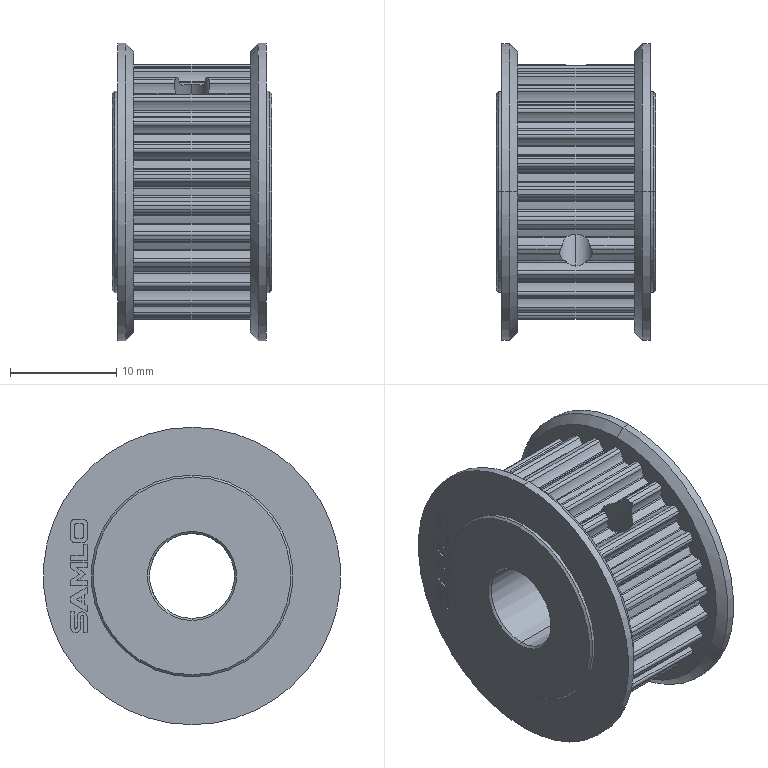Part | STEP file | TAAS3M_26_100_P8 | 1 solid | 320 faces | box 15 x 28 x 28 mm | volume 5701 mm3 | cylinder 250 | plane 58 | cone 12 | commonest cylinder face diameters 0.3 x57 0.56 x56 3.95 x56 21.85 x28 24.07 x27 0.362 x4